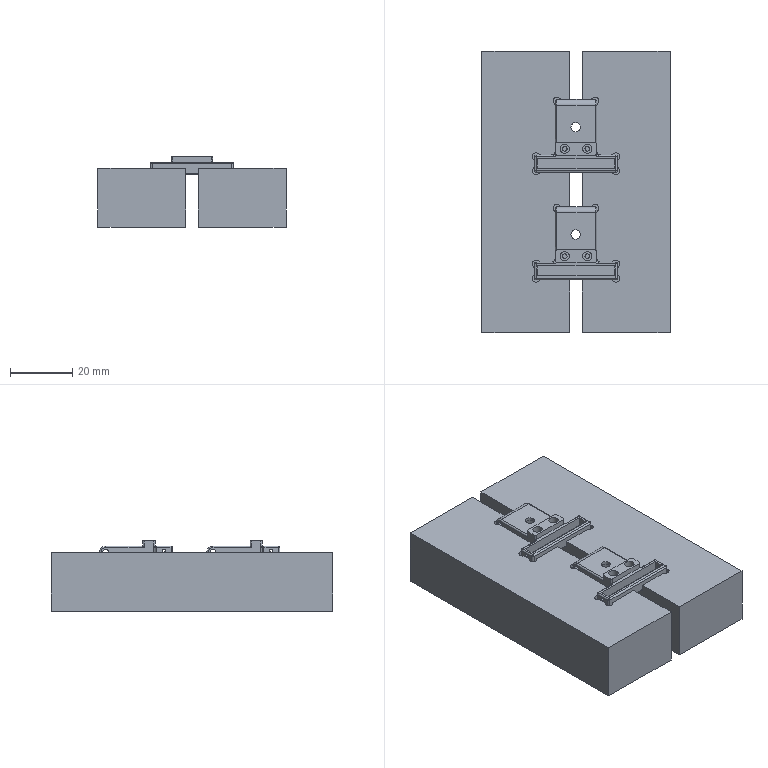CAM job | NX | 3-axis milling, drilling | part box 60.696 x 90.669 x 22.754 mm
Tools:
number,name,description,diameter,corner_radius,flute_length,length,flutes
17,D2,平底铣刀-粗,2.0,0.0,50.0,75.0,2
3,D3,平底铣刀-粗,3.0,0.0,20.0,75.0,2
4,D4,平底铣刀-粗,4.0,0.0,25.0,75.0,2
6,D6,平底铣刀-粗,6.0,0.0,25.0,75.0,2
9,D10,平底铣刀-粗,10.0,0.0,35.0,75.0,2
19,D2-J,平底铣刀-精,2.0,0.0,50.0,75.0,2
11,D3-J,平底铣刀-精,3.0,0.0,50.0,75.0,2
7,D6-J,平底铣刀-精,6.0,0.0,25.0,75.0,2
20,D4R0.5,圆鼻刀-粗,4.0,0.5,50.0,75.0,2
1,D80R0.8飞刀,圆鼻刀-粗,80.0,0.8,50.0,75.0,2
2,D6倒角刀,倒角刀,6.0,0.0,3.0,25.0,2
23,ZT1,钻头,1.0,0.0,35.0,50.0,2
17,ZT1.5,钻头,1.5,0.0,35.0,50.0,2
18,ZT3,钻头,3.0,0.0,35.0,50.0,2
Operations:
program,operation,operation_type,tool,method,geometry_group,spindle_rpm,surface_speed,feed_per_tooth,feed_cut,feed_plunge,cut_length_mm,path_length_mm,cut_time_min,machine_time_min
C,底壁铣分层开粗-中_COPY_1,VolumeBased25DMillingOperation,D4,分层开粗-切深K-步距G,W-C,8000.0,100.528,0.125,2000.0,100.0,2494.652,2598.285,1.247,1.258
C,等高光顺清角D2参考6_COPY,ZLevelMilling,D2-J,分层精光-切深K-步距G,W-C,8000.0,50.264,0.05,800.0,100.0,1788.805,2591.452,2.236,2.316
C,底壁铣精光底面-中_COPY_2,VolumeBased25DMillingOperation,D2-J,精光步距切深关,W-C,7000.0,175.0,0.0536,1500.0,100.0,643.858,711.843,0.4292,0.436
C,平面去毛刺6X45L_COPY_1,SurfaceContour,D6倒角刀,爬面_倒角-切深0-步距G,W-C,6500.0,122.519,0.1154,1500.0,100.0,201.481,464.529,0.1343,0.1606
C,底壁铣精光侧面-中-选底面_COPY,VolumeBased25DMillingOperation,D2-J,侧刃精光-切深K-步距G,W-C,8000.0,100.528,0.05,800.0,100.0,211.469,290.047,0.2643,0.2722
B,动态开粗D10_COPY,CavityMilling,D10,动态开粗-切深K-步距K,W-B,8000.0,251.32,0.25,4000.0,100.0,3587.695,3623.495,0.8969,0.9005
B,底壁铣分层开粗-中_COPY,VolumeBased25DMillingOperation,D6,分层开粗-切深K-步距G,W-B,8000.0,150.792,0.1875,3000.0,100.0,2309.763,3166.273,0.7699,0.8556
B,等高精光往复爬面_COPY_COPY_COPY_COPY,ZLevelMilling,D6,等高爬面-切深K-步距G,W-B,9000.0,84.823,0.25,4500.0,100.0,893.48,989.009,0.1986,0.2081
B,底壁铣螺旋开粗-小_COPY,VolumeBased25DMillingOperation,D2,分层开粗-切深K-步距G,W-B,8000.0,50.264,0.0938,1500.0,100.0,2965.316,3093.247,1.977,1.99
B,底壁铣螺旋开粗-小_COPY_1,VolumeBased25DMillingOperation,D2,分层开粗-切深K-步距G,W-B,8000.0,50.264,0.0312,500.0,100.0,416.719,632.964,0.8334,0.8551
B,底壁铣螺旋精光-小_COPY,VolumeBased25DMillingOperation,D2-J,螺旋精光-切深K-步距G,W-B,8000.0,50.266,0.05,800.0,100.0,403.894,531.07,0.5049,0.5176
B,底壁铣精光底面-中_COPY_1,VolumeBased25DMillingOperation,D6-J,精光步距切深关,W-B,7000.0,175.0,0.0536,1500.0,100.0,92.268,154.423,0.0615,0.0677
B,底壁铣精光底面-中_COPY,VolumeBased25DMillingOperation,D6-J,精光步距切深关,W-B,7000.0,175.0,0.0536,1500.0,100.0,345.112,498.437,0.2301,0.2454
B,等高精光往复爬面_COPY_COPY_COPY_1,ZLevelMilling,D4R0.5,等高爬面-切深K-步距G,W-B,9000.0,84.823,0.25,4500.0,100.0,1843.156,1942.345,0.4096,0.4195
B,打点,Operation,D6倒角刀,METHOD,W-B,8000.0,150.796,0.1562,2500.0,0.0,8.0,108.287,0.0032,0.0132
B,钻倒角_2,Operation,D6倒角刀,METHOD,W-B,8000.0,150.796,0.0625,1000.0,0.0,9.6,100.438,0.0096,0.0187
B,钻倒角_3,Operation,D6倒角刀,METHOD,W-B,8000.0,150.796,0.0625,1000.0,0.0,19.2,137.855,0.0192,0.0311
B,平面去毛刺6X45L_COPY,SurfaceContour,D6倒角刀,爬面_倒角-切深0-步距G,W-B,6500.0,122.519,0.1154,1500.0,100.0,216.782,492.396,0.1445,0.1721
B,底壁铣螺旋精光-小_COPY_1,VolumeBased25DMillingOperation,D2-J,螺旋精光-切深K-步距G,W-B,8000.0,50.266,0.0125,200.0,100.0,97.627,312.318,0.4881,0.5096
B,等高精光-中_COPY,ZLevelMilling,D6-J,侧刃精光-切深K-步距G,W-B,8000.0,150.792,0.0625,1000.0,100.0,113.963,211.395,0.114,0.1237
B,等高精光往复爬面_COPY_COPY_COPY_1_COPY,ZLevelMilling,D6-J,等高爬面-切深K-步距G,W-B,9000.0,84.823,0.25,4500.0,100.0,2363.303,2575.739,0.5252,0.5464
B,等高精光往复爬面_COPY_COPY_COPY_1_COPY_COPY,ZLevelMilling,D6-J,等高爬面-切深K-步距G,W-B,9000.0,84.823,0.25,4500.0,100.0,5764.097,5851.091,1.281,1.29
A,顶面,FaceMilling,D80R0.8飞刀,侧刃精光-切深K-步距G,W-A,4000.0,1005.31,0.125,1000.0,100.0,152.169,188.169,0.1522,0.1558
A,外形粗_2,VolumeBased25DMillingOperation,D10,METHOD,W-A,8000.0,251.327,0.3125,5000.0,80.0,2541.211,2664.723,0.5082,0.5206
A,等高精光往复爬面_COPY_COPY_COPY,ZLevelMilling,D10,等高爬面-切深K-步距G,W-A,9000.0,84.823,0.25,4500.0,100.0,1309.017,1395.054,0.2909,0.2995
A,打点-深0.8,Operation,D6倒角刀,NONE,W-A,8000.0,150.796,0.0312,500.0,90.0,13.6,194.81,0.0272,0.0453
A,G83钻孔4.2L_COPY,Operation,ZT1,钻孔-切深G-步距G,W-A,5000.0,15.708,0.002,20.0,100.0,6.0,87.614,0.3,0.3082
A,通孔-1-2,Operation,ZT1.5,NONE,W-A,3000.0,14.137,0.005,30.0,90.0,36.0,164.287,1.2,1.213
A,沉头孔-钻孔0段,Operation,ZT3,NONE,W-A,2800.0,26.389,0.0179,100.0,90.0,15.803,107.22,0.158,0.1672
A,铣孔开粗D4_1,CylinderMilling,D3,NONE,W-A,8000.0,100.531,0.075,1200.0,100.0,149.097,268.697,0.1242,0.1362
A,外形侧面,ZLevelMilling,D2-J,METHOD,W-A,9000.0,84.823,0.1389,2500.0,80.0,1113.497,1367.957,0.4457,0.4711
A,等高精光往复爬面_COPY,ZLevelMilling,D4R0.5,等高爬面-切深K-步距G,W-A,9000.0,84.823,0.25,4500.0,100.0,2665.8,2749.281,0.5924,0.6007
A,等高精光往复爬面_COPY_COPY,ZLevelMilling,D4R0.5,等高爬面-切深K-步距G,W-A,9000.0,84.823,0.25,4500.0,100.0,1791.674,1873.531,0.3981,0.4063
A,钻倒角_1,Operation,D6倒角刀,METHOD,W-A,8000.0,150.796,0.0312,500.0,0.0,16.2,131.855,0.0324,0.044
A,铣倒角_1,PlanarMilling,D6倒角刀,NONE,W-A,8000.0,150.796,0.0312,500.0,100.0,49.086,154.728,0.0982,0.1087
A,底壁铣精光侧面-中_COPY,VolumeBased25DMillingOperation,D3-J,侧刃精光-切深K-步距G,W-A,8000.0,75.398,0.0312,500.0,100.0,24.026,105.497,0.0481,0.0562
A,外形半精_2,VolumeBased25DMillingOperation,D6-J,METHOD,W-A,8000.0,251.327,0.0625,1000.0,100.0,240.894,377.289,0.2409,0.2545